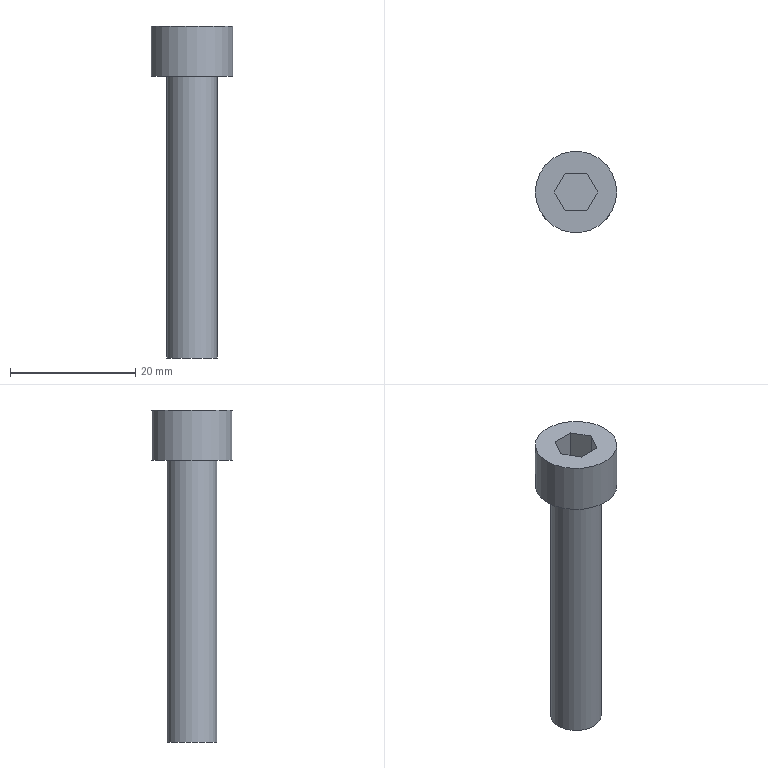Part | STEP file | 1 solid | 12 faces | box 13 x 13 x 53 mm | volume 3159 mm3 | plane 10 | cylinder 2 | commonest cylinder face diameters 8 x1 13 x1
STEP:
#1=CARTESIAN_POINT('',(0.,0.,0.));
#2=DIRECTION('',(0.,0.,1.));
#3=DIRECTION('',(1.,0.,0.));
#4=AXIS2_PLACEMENT_3D('',#1,#2,#3);
#5=CARTESIAN_POINT('',(1566.747,387.48,-61.381));
#6=VERTEX_POINT('',#5);
#7=CARTESIAN_POINT('',(1560.247,387.48,-61.381));
#8=DIRECTION('',(0.,0.,1.));
#9=DIRECTION('',(1.,0.,0.));
#10=AXIS2_PLACEMENT_3D('',#7,#8,#9);
#11=CIRCLE('',#10,6.5);
#12=CARTESIAN_POINT('',(1566.747,387.48,-61.381));
#13=DIRECTION('',(0.,0.,-1.));
#14=DIRECTION('',(-1.,0.,0.));
#15=AXIS2_PLACEMENT_3D('',#12,#13,#14);
#16=PLANE('',#15);
#17=CARTESIAN_POINT('',(0.,0.));
#18=CARTESIAN_POINT('',(0.,11.258));
#19=CARTESIAN_POINT('',(9.75,5.629));
#20=CARTESIAN_POINT('',(19.5,0.));
#21=CARTESIAN_POINT('',(9.75,-5.629));
#22=CARTESIAN_POINT('',(0.,-11.258));
#23=CARTESIAN_POINT('',(0.,0.));
#24=(BOUNDED_CURVE()B_SPLINE_CURVE(2,(#17,#18,#19,#20,#21,#22,#23),.UNSPECIFIED.,.T.,.F.)B_SPLINE_CURVE_WITH_KNOTS((1,2,2,2,2,1),(-2.094,0.,2.094,4.189,6.283,8.378),.UNSPECIFIED.)CURVE()GEOMETRIC_REPRESENTATION_ITEM()RATIONAL_B_SPLINE_CURVE((1.,0.5,1.,0.5,1.,0.5,1.))REPRESENTATION_ITEM(''));
#25=(GEOMETRIC_REPRESENTATION_CONTEXT(2)PARAMETRIC_REPRESENTATION_CONTEXT()REPRESENTATION_CONTEXT('',''));
#26=DEFINITIONAL_REPRESENTATION('',(#24),#25);
#27=PCURVE('',#16,#26);
#28=CARTESIAN_POINT('',(1560.247,387.48,-101.281));
#29=DIRECTION('',(0.,0.,1.));
#30=DIRECTION('',(1.,0.,0.));
#31=AXIS2_PLACEMENT_3D('',#28,#29,#30);
#32=CYLINDRICAL_SURFACE('',#31,6.5);
#33=CARTESIAN_POINT('',(0.,39.9));
#34=DIRECTION('',(1.,0.));
#35=VECTOR('',#34,1.);
#36=LINE('',#33,#35);
#37=(GEOMETRIC_REPRESENTATION_CONTEXT(2)PARAMETRIC_REPRESENTATION_CONTEXT()REPRESENTATION_CONTEXT('',''));
#38=DEFINITIONAL_REPRESENTATION('',(#36),#37);
#39=PCURVE('',#32,#38);
#40=SURFACE_CURVE('',#11,(#27,#39),.PCURVE_S1.);
#41=EDGE_CURVE('',#6,#6,#40,.T.);
#42=ORIENTED_EDGE('',*,*,#41,.T.);
#43=EDGE_LOOP('',(#42));
#44=FACE_BOUND('',#43,.T.);
#45=CARTESIAN_POINT('',(1558.515,390.48,-61.381));
#46=VERTEX_POINT('',#45);
#47=CARTESIAN_POINT('',(1561.979,390.48,-61.381));
#48=VERTEX_POINT('',#47);
#49=CARTESIAN_POINT('',(1558.515,390.48,-61.381));
#50=DIRECTION('',(1.,0.,0.));
#51=VECTOR('',#50,1.);
#52=LINE('',#49,#51);
#53=CARTESIAN_POINT('',(8.232,3.));
#54=DIRECTION('',(-1.,0.));
#55=VECTOR('',#54,1.);
#56=LINE('',#53,#55);
#57=(GEOMETRIC_REPRESENTATION_CONTEXT(2)PARAMETRIC_REPRESENTATION_CONTEXT()REPRESENTATION_CONTEXT('',''));
#58=DEFINITIONAL_REPRESENTATION('',(#56),#57);
#59=PCURVE('',#16,#58);
#60=CARTESIAN_POINT('',(1558.515,390.48,-66.661));
#61=DIRECTION('',(0.,-1.,0.));
#62=DIRECTION('',(1.,0.,0.));
#63=AXIS2_PLACEMENT_3D('',#60,#61,#62);
#64=PLANE('',#63);
#65=CARTESIAN_POINT('',(0.,5.28));
#66=DIRECTION('',(1.,0.));
#67=VECTOR('',#66,1.);
#68=LINE('',#65,#67);
#69=(GEOMETRIC_REPRESENTATION_CONTEXT(2)PARAMETRIC_REPRESENTATION_CONTEXT()REPRESENTATION_CONTEXT('',''));
#70=DEFINITIONAL_REPRESENTATION('',(#68),#69);
#71=PCURVE('',#64,#70);
#72=SURFACE_CURVE('',#52,(#59,#71),.PCURVE_S1.);
#73=EDGE_CURVE('',#46,#48,#72,.T.);
#74=ORIENTED_EDGE('',*,*,#73,.T.);
#75=CARTESIAN_POINT('',(1563.711,387.48,-61.381));
#76=VERTEX_POINT('',#75);
#77=CARTESIAN_POINT('',(1561.979,390.48,-61.381));
#78=DIRECTION('',(0.5,-0.866,0.));
#79=VECTOR('',#78,1.);
#80=LINE('',#77,#79);
#81=CARTESIAN_POINT('',(4.768,3.));
#82=DIRECTION('',(-0.5,-0.866));
#83=VECTOR('',#82,1.);
#84=LINE('',#81,#83);
#85=(GEOMETRIC_REPRESENTATION_CONTEXT(2)PARAMETRIC_REPRESENTATION_CONTEXT()REPRESENTATION_CONTEXT('',''));
#86=DEFINITIONAL_REPRESENTATION('',(#84),#85);
#87=PCURVE('',#16,#86);
#88=CARTESIAN_POINT('',(1561.979,390.48,-66.661));
#89=DIRECTION('',(-0.866,-0.5,0.));
#90=DIRECTION('',(0.5,-0.866,0.));
#91=AXIS2_PLACEMENT_3D('',#88,#89,#90);
#92=PLANE('',#91);
#93=CARTESIAN_POINT('',(0.,5.28));
#94=DIRECTION('',(1.,0.));
#95=VECTOR('',#94,1.);
#96=LINE('',#93,#95);
#97=(GEOMETRIC_REPRESENTATION_CONTEXT(2)PARAMETRIC_REPRESENTATION_CONTEXT()REPRESENTATION_CONTEXT('',''));
#98=DEFINITIONAL_REPRESENTATION('',(#96),#97);
#99=PCURVE('',#92,#98);
#100=SURFACE_CURVE('',#80,(#87,#99),.PCURVE_S1.);
#101=EDGE_CURVE('',#48,#76,#100,.T.);
#102=ORIENTED_EDGE('',*,*,#101,.T.);
#103=CARTESIAN_POINT('',(1561.979,384.48,-61.381));
#104=VERTEX_POINT('',#103);
#105=CARTESIAN_POINT('',(1563.711,387.48,-61.381));
#106=DIRECTION('',(-0.5,-0.866,0.));
#107=VECTOR('',#106,1.);
#108=LINE('',#105,#107);
#109=CARTESIAN_POINT('',(3.036,0.));
#110=DIRECTION('',(0.5,-0.866));
#111=VECTOR('',#110,1.);
#112=LINE('',#109,#111);
#113=(GEOMETRIC_REPRESENTATION_CONTEXT(2)PARAMETRIC_REPRESENTATION_CONTEXT()REPRESENTATION_CONTEXT('',''));
#114=DEFINITIONAL_REPRESENTATION('',(#112),#113);
#115=PCURVE('',#16,#114);
#116=CARTESIAN_POINT('',(1563.711,387.48,-66.661));
#117=DIRECTION('',(-0.866,0.5,0.));
#118=DIRECTION('',(-0.5,-0.866,0.));
#119=AXIS2_PLACEMENT_3D('',#116,#117,#118);
#120=PLANE('',#119);
#121=CARTESIAN_POINT('',(0.,5.28));
#122=DIRECTION('',(1.,0.));
#123=VECTOR('',#122,1.);
#124=LINE('',#121,#123);
#125=(GEOMETRIC_REPRESENTATION_CONTEXT(2)PARAMETRIC_REPRESENTATION_CONTEXT()REPRESENTATION_CONTEXT('',''));
#126=DEFINITIONAL_REPRESENTATION('',(#124),#125);
#127=PCURVE('',#120,#126);
#128=SURFACE_CURVE('',#108,(#115,#127),.PCURVE_S1.);
#129=EDGE_CURVE('',#76,#104,#128,.T.);
#130=ORIENTED_EDGE('',*,*,#129,.T.);
#131=CARTESIAN_POINT('',(1558.515,384.48,-61.381));
#132=VERTEX_POINT('',#131);
#133=CARTESIAN_POINT('',(1561.979,384.48,-61.381));
#134=DIRECTION('',(-1.,0.,0.));
#135=VECTOR('',#134,1.);
#136=LINE('',#133,#135);
#137=CARTESIAN_POINT('',(4.768,-3.));
#138=DIRECTION('',(1.,0.));
#139=VECTOR('',#138,1.);
#140=LINE('',#137,#139);
#141=(GEOMETRIC_REPRESENTATION_CONTEXT(2)PARAMETRIC_REPRESENTATION_CONTEXT()REPRESENTATION_CONTEXT('',''));
#142=DEFINITIONAL_REPRESENTATION('',(#140),#141);
#143=PCURVE('',#16,#142);
#144=CARTESIAN_POINT('',(1561.979,384.48,-66.661));
#145=DIRECTION('',(0.,1.,0.));
#146=DIRECTION('',(-1.,0.,0.));
#147=AXIS2_PLACEMENT_3D('',#144,#145,#146);
#148=PLANE('',#147);
#149=CARTESIAN_POINT('',(0.,5.28));
#150=DIRECTION('',(1.,0.));
#151=VECTOR('',#150,1.);
#152=LINE('',#149,#151);
#153=(GEOMETRIC_REPRESENTATION_CONTEXT(2)PARAMETRIC_REPRESENTATION_CONTEXT()REPRESENTATION_CONTEXT('',''));
#154=DEFINITIONAL_REPRESENTATION('',(#152),#153);
#155=PCURVE('',#148,#154);
#156=SURFACE_CURVE('',#136,(#143,#155),.PCURVE_S1.);
#157=EDGE_CURVE('',#104,#132,#156,.T.);
#158=ORIENTED_EDGE('',*,*,#157,.T.);
#159=CARTESIAN_POINT('',(1556.783,387.48,-61.381));
#160=VERTEX_POINT('',#159);
#161=CARTESIAN_POINT('',(1558.515,384.48,-61.381));
#162=DIRECTION('',(-0.5,0.866,0.));
#163=VECTOR('',#162,1.);
#164=LINE('',#161,#163);
#165=CARTESIAN_POINT('',(8.232,-3.));
#166=DIRECTION('',(0.5,0.866));
#167=VECTOR('',#166,1.);
#168=LINE('',#165,#167);
#169=(GEOMETRIC_REPRESENTATION_CONTEXT(2)PARAMETRIC_REPRESENTATION_CONTEXT()REPRESENTATION_CONTEXT('',''));
#170=DEFINITIONAL_REPRESENTATION('',(#168),#169);
#171=PCURVE('',#16,#170);
#172=CARTESIAN_POINT('',(1558.515,384.48,-66.661));
#173=DIRECTION('',(0.866,0.5,0.));
#174=DIRECTION('',(-0.5,0.866,0.));
#175=AXIS2_PLACEMENT_3D('',#172,#173,#174);
#176=PLANE('',#175);
#177=CARTESIAN_POINT('',(0.,5.28));
#178=DIRECTION('',(1.,0.));
#179=VECTOR('',#178,1.);
#180=LINE('',#177,#179);
#181=(GEOMETRIC_REPRESENTATION_CONTEXT(2)PARAMETRIC_REPRESENTATION_CONTEXT()REPRESENTATION_CONTEXT('',''));
#182=DEFINITIONAL_REPRESENTATION('',(#180),#181);
#183=PCURVE('',#176,#182);
#184=SURFACE_CURVE('',#164,(#171,#183),.PCURVE_S1.);
#185=EDGE_CURVE('',#132,#160,#184,.T.);
#186=ORIENTED_EDGE('',*,*,#185,.T.);
#187=CARTESIAN_POINT('',(1556.783,387.48,-61.381));
#188=DIRECTION('',(0.5,0.866,0.));
#189=VECTOR('',#188,1.);
#190=LINE('',#187,#189);
#191=CARTESIAN_POINT('',(9.964,0.));
#192=DIRECTION('',(-0.5,0.866));
#193=VECTOR('',#192,1.);
#194=LINE('',#191,#193);
#195=(GEOMETRIC_REPRESENTATION_CONTEXT(2)PARAMETRIC_REPRESENTATION_CONTEXT()REPRESENTATION_CONTEXT('',''));
#196=DEFINITIONAL_REPRESENTATION('',(#194),#195);
#197=PCURVE('',#16,#196);
#198=CARTESIAN_POINT('',(1556.783,387.48,-66.661));
#199=DIRECTION('',(0.866,-0.5,0.));
#200=DIRECTION('',(0.5,0.866,0.));
#201=AXIS2_PLACEMENT_3D('',#198,#199,#200);
#202=PLANE('',#201);
#203=CARTESIAN_POINT('',(0.,5.28));
#204=DIRECTION('',(1.,0.));
#205=VECTOR('',#204,1.);
#206=LINE('',#203,#205);
#207=(GEOMETRIC_REPRESENTATION_CONTEXT(2)PARAMETRIC_REPRESENTATION_CONTEXT()REPRESENTATION_CONTEXT('',''));
#208=DEFINITIONAL_REPRESENTATION('',(#206),#207);
#209=PCURVE('',#202,#208);
#210=SURFACE_CURVE('',#190,(#197,#209),.PCURVE_S1.);
#211=EDGE_CURVE('',#160,#46,#210,.T.);
#212=ORIENTED_EDGE('',*,*,#211,.T.);
#213=EDGE_LOOP('',(#74,#102,#130,#158,#186,#212));
#214=FACE_BOUND('',#213,.T.);
#215=ADVANCED_FACE('',(#44,#214),#16,.F.);
#216=ORIENTED_EDGE('',*,*,#41,.F.);
#217=CARTESIAN_POINT('',(1566.747,387.48,-69.381));
#218=VERTEX_POINT('',#217);
#219=CARTESIAN_POINT('',(1566.747,387.48,-69.381));
#220=CARTESIAN_POINT('',(1566.747,387.48,-61.381));
#221=B_SPLINE_CURVE_WITH_KNOTS('',1,(#219,#220),.UNSPECIFIED.,.F.,.F.,(2,2),(31.9,39.9),.PIECEWISE_BEZIER_KNOTS.);
#222=CARTESIAN_POINT('',(0.,0.));
#223=DIRECTION('',(0.,1.));
#224=VECTOR('',#223,1.);
#225=LINE('',#222,#224);
#226=(GEOMETRIC_REPRESENTATION_CONTEXT(2)PARAMETRIC_REPRESENTATION_CONTEXT()REPRESENTATION_CONTEXT('',''));
#227=DEFINITIONAL_REPRESENTATION('',(#225),#226);
#228=PCURVE('',#32,#227);
#229=CARTESIAN_POINT('',(6.283,0.));
#230=DIRECTION('',(0.,1.));
#231=VECTOR('',#230,1.);
#232=LINE('',#229,#231);
#233=(GEOMETRIC_REPRESENTATION_CONTEXT(2)PARAMETRIC_REPRESENTATION_CONTEXT()REPRESENTATION_CONTEXT('',''));
#234=DEFINITIONAL_REPRESENTATION('',(#232),#233);
#235=PCURVE('',#32,#234);
#236=SEAM_CURVE('',#221,(#228,#235),.PCURVE_S1.);
#237=EDGE_CURVE('',#218,#6,#236,.T.);
#238=ORIENTED_EDGE('',*,*,#237,.F.);
#239=CARTESIAN_POINT('',(1560.247,387.48,-69.381));
#240=DIRECTION('',(0.,0.,1.));
#241=DIRECTION('',(1.,0.,0.));
#242=AXIS2_PLACEMENT_3D('',#239,#240,#241);
#243=CIRCLE('',#242,6.5);
#244=CARTESIAN_POINT('',(0.,31.9));
#245=DIRECTION('',(1.,0.));
#246=VECTOR('',#245,1.);
#247=LINE('',#244,#246);
#248=(GEOMETRIC_REPRESENTATION_CONTEXT(2)PARAMETRIC_REPRESENTATION_CONTEXT()REPRESENTATION_CONTEXT('',''));
#249=DEFINITIONAL_REPRESENTATION('',(#247),#248);
#250=PCURVE('',#32,#249);
#251=CARTESIAN_POINT('',(1564.247,387.48,-69.381));
#252=DIRECTION('',(0.,0.,1.));
#253=DIRECTION('',(1.,0.,0.));
#254=AXIS2_PLACEMENT_3D('',#251,#252,#253);
#255=PLANE('',#254);
#256=CARTESIAN_POINT('',(-4.,0.));
#257=DIRECTION('',(1.,0.));
#258=AXIS2_PLACEMENT_2D('',#256,#257);
#259=CIRCLE('',#258,6.5);
#260=(GEOMETRIC_REPRESENTATION_CONTEXT(2)PARAMETRIC_REPRESENTATION_CONTEXT()REPRESENTATION_CONTEXT('',''));
#261=DEFINITIONAL_REPRESENTATION('',(#259),#260);
#262=PCURVE('',#255,#261);
#263=SURFACE_CURVE('',#243,(#250,#262),.PCURVE_S1.);
#264=EDGE_CURVE('',#218,#218,#263,.T.);
#265=ORIENTED_EDGE('',*,*,#264,.T.);
#266=ORIENTED_EDGE('',*,*,#237,.T.);
#267=EDGE_LOOP('',(#216,#238,#265,#266));
#268=FACE_BOUND('',#267,.T.);
#269=ADVANCED_FACE('',(#268),#32,.T.);
#270=ORIENTED_EDGE('',*,*,#264,.F.);
#271=EDGE_LOOP('',(#270));
#272=FACE_BOUND('',#271,.T.);
#273=CARTESIAN_POINT('',(1564.247,387.48,-69.381));
#274=VERTEX_POINT('',#273);
#275=CARTESIAN_POINT('',(1560.247,387.48,-69.381));
#276=DIRECTION('',(0.,0.,1.));
#277=DIRECTION('',(1.,0.,0.));
#278=AXIS2_PLACEMENT_3D('',#275,#276,#277);
#279=CIRCLE('',#278,4.);
#280=CARTESIAN_POINT('',(-4.,0.));
#281=DIRECTION('',(1.,0.));
#282=AXIS2_PLACEMENT_2D('',#280,#281);
#283=CIRCLE('',#282,4.);
#284=(GEOMETRIC_REPRESENTATION_CONTEXT(2)PARAMETRIC_REPRESENTATION_CONTEXT()REPRESENTATION_CONTEXT('',''));
#285=DEFINITIONAL_REPRESENTATION('',(#283),#284);
#286=PCURVE('',#255,#285);
#287=CARTESIAN_POINT('',(1560.247,387.48,-101.281));
#288=DIRECTION('',(0.,0.,1.));
#289=DIRECTION('',(1.,0.,0.));
#290=AXIS2_PLACEMENT_3D('',#287,#288,#289);
#291=CYLINDRICAL_SURFACE('',#290,4.);
#292=CARTESIAN_POINT('',(0.,31.9));
#293=DIRECTION('',(1.,0.));
#294=VECTOR('',#293,1.);
#295=LINE('',#292,#294);
#296=(GEOMETRIC_REPRESENTATION_CONTEXT(2)PARAMETRIC_REPRESENTATION_CONTEXT()REPRESENTATION_CONTEXT('',''));
#297=DEFINITIONAL_REPRESENTATION('',(#295),#296);
#298=PCURVE('',#291,#297);
#299=SURFACE_CURVE('',#279,(#286,#298),.PCURVE_S1.);
#300=EDGE_CURVE('',#274,#274,#299,.T.);
#301=ORIENTED_EDGE('',*,*,#300,.T.);
#302=EDGE_LOOP('',(#301));
#303=FACE_BOUND('',#302,.T.);
#304=ADVANCED_FACE('',(#272,#303),#255,.F.);
#305=ORIENTED_EDGE('',*,*,#300,.F.);
#306=CARTESIAN_POINT('',(1564.247,387.48,-114.381));
#307=VERTEX_POINT('',#306);
#308=CARTESIAN_POINT('',(1564.247,387.48,-114.381));
#309=CARTESIAN_POINT('',(1564.247,387.48,-69.381));
#310=B_SPLINE_CURVE_WITH_KNOTS('',1,(#308,#309),.UNSPECIFIED.,.F.,.F.,(2,2),(-13.1,31.9),.PIECEWISE_BEZIER_KNOTS.);
#311=CARTESIAN_POINT('',(0.,0.));
#312=DIRECTION('',(0.,1.));
#313=VECTOR('',#312,1.);
#314=LINE('',#311,#313);
#315=(GEOMETRIC_REPRESENTATION_CONTEXT(2)PARAMETRIC_REPRESENTATION_CONTEXT()REPRESENTATION_CONTEXT('',''));
#316=DEFINITIONAL_REPRESENTATION('',(#314),#315);
#317=PCURVE('',#291,#316);
#318=CARTESIAN_POINT('',(6.283,0.));
#319=DIRECTION('',(0.,1.));
#320=VECTOR('',#319,1.);
#321=LINE('',#318,#320);
#322=(GEOMETRIC_REPRESENTATION_CONTEXT(2)PARAMETRIC_REPRESENTATION_CONTEXT()REPRESENTATION_CONTEXT('',''));
#323=DEFINITIONAL_REPRESENTATION('',(#321),#322);
#324=PCURVE('',#291,#323);
#325=SEAM_CURVE('',#310,(#317,#324),.PCURVE_S1.);
#326=EDGE_CURVE('',#307,#274,#325,.T.);
#327=ORIENTED_EDGE('',*,*,#326,.F.);
#328=CARTESIAN_POINT('',(1560.247,387.48,-114.381));
#329=DIRECTION('',(0.,0.,1.));
#330=DIRECTION('',(1.,0.,0.));
#331=AXIS2_PLACEMENT_3D('',#328,#329,#330);
#332=CIRCLE('',#331,4.);
#333=CARTESIAN_POINT('',(0.,-13.1));
#334=DIRECTION('',(1.,0.));
#335=VECTOR('',#334,1.);
#336=LINE('',#333,#335);
#337=(GEOMETRIC_REPRESENTATION_CONTEXT(2)PARAMETRIC_REPRESENTATION_CONTEXT()REPRESENTATION_CONTEXT('',''));
#338=DEFINITIONAL_REPRESENTATION('',(#336),#337);
#339=PCURVE('',#291,#338);
#340=CARTESIAN_POINT('',(1560.247,387.48,-114.381));
#341=DIRECTION('',(0.,0.,1.));
#342=DIRECTION('',(1.,0.,0.));
#343=AXIS2_PLACEMENT_3D('',#340,#341,#342);
#344=PLANE('',#343);
#345=CARTESIAN_POINT('',(0.,0.));
#346=DIRECTION('',(1.,0.));
#347=AXIS2_PLACEMENT_2D('',#345,#346);
#348=CIRCLE('',#347,4.);
#349=(GEOMETRIC_REPRESENTATION_CONTEXT(2)PARAMETRIC_REPRESENTATION_CONTEXT()REPRESENTATION_CONTEXT('',''));
#350=DEFINITIONAL_REPRESENTATION('',(#348),#349);
#351=PCURVE('',#344,#350);
#352=SURFACE_CURVE('',#332,(#339,#351),.PCURVE_S1.);
#353=EDGE_CURVE('',#307,#307,#352,.T.);
#354=ORIENTED_EDGE('',*,*,#353,.T.);
#355=ORIENTED_EDGE('',*,*,#326,.T.);
#356=EDGE_LOOP('',(#305,#327,#354,#355));
#357=FACE_BOUND('',#356,.T.);
#358=ADVANCED_FACE('',(#357),#291,.T.);
#359=ORIENTED_EDGE('',*,*,#353,.F.);
#360=EDGE_LOOP('',(#359));
#361=FACE_BOUND('',#360,.T.);
#362=ADVANCED_FACE('',(#361),#344,.F.);
#363=ORIENTED_EDGE('',*,*,#73,.F.);
#364=CARTESIAN_POINT('',(1558.515,390.48,-66.661));
#365=VERTEX_POINT('',#364);
#366=CARTESIAN_POINT('',(1558.515,390.48,-66.661));
#367=DIRECTION('',(0.,0.,-1.));
#368=VECTOR('',#367,1.);
#369=LINE('',#366,#368);
#370=CARTESIAN_POINT('',(0.,0.));
#371=DIRECTION('',(0.,-1.));
#372=VECTOR('',#371,1.);
#373=LINE('',#370,#372);
#374=(GEOMETRIC_REPRESENTATION_CONTEXT(2)PARAMETRIC_REPRESENTATION_CONTEXT()REPRESENTATION_CONTEXT('',''));
#375=DEFINITIONAL_REPRESENTATION('',(#373),#374);
#376=PCURVE('',#64,#375);
#377=CARTESIAN_POINT('',(3.464,0.));
#378=DIRECTION('',(0.,-1.));
#379=VECTOR('',#378,1.);
#380=LINE('',#377,#379);
#381=(GEOMETRIC_REPRESENTATION_CONTEXT(2)PARAMETRIC_REPRESENTATION_CONTEXT()REPRESENTATION_CONTEXT('',''));
#382=DEFINITIONAL_REPRESENTATION('',(#380),#381);
#383=PCURVE('',#202,#382);
#384=SURFACE_CURVE('',#369,(#376,#383),.PCURVE_S1.);
#385=EDGE_CURVE('',#46,#365,#384,.T.);
#386=ORIENTED_EDGE('',*,*,#385,.T.);
#387=CARTESIAN_POINT('',(1561.979,390.48,-66.661));
#388=VERTEX_POINT('',#387);
#389=CARTESIAN_POINT('',(1558.515,390.48,-66.661));
#390=DIRECTION('',(-1.,0.,0.));
#391=VECTOR('',#390,1.);
#392=LINE('',#389,#391);
#393=CARTESIAN_POINT('',(0.,0.));
#394=DIRECTION('',(-1.,0.));
#395=VECTOR('',#394,1.);
#396=LINE('',#393,#395);
#397=(GEOMETRIC_REPRESENTATION_CONTEXT(2)PARAMETRIC_REPRESENTATION_CONTEXT()REPRESENTATION_CONTEXT('',''));
#398=DEFINITIONAL_REPRESENTATION('',(#396),#397);
#399=PCURVE('',#64,#398);
#400=CARTESIAN_POINT('',(1560.247,387.48,-66.661));
#401=DIRECTION('',(0.,0.,-1.));
#402=DIRECTION('',(-1.,0.,0.));
#403=AXIS2_PLACEMENT_3D('',#400,#401,#402);
#404=PLANE('',#403);
#405=CARTESIAN_POINT('',(1.732,3.));
#406=DIRECTION('',(1.,0.));
#407=VECTOR('',#406,1.);
#408=LINE('',#405,#407);
#409=(GEOMETRIC_REPRESENTATION_CONTEXT(2)PARAMETRIC_REPRESENTATION_CONTEXT()REPRESENTATION_CONTEXT('',''));
#410=DEFINITIONAL_REPRESENTATION('',(#408),#409);
#411=PCURVE('',#404,#410);
#412=SURFACE_CURVE('',#392,(#399,#411),.PCURVE_S1.);
#413=EDGE_CURVE('',#388,#365,#412,.T.);
#414=ORIENTED_EDGE('',*,*,#413,.F.);
#415=CARTESIAN_POINT('',(1561.979,390.48,-66.661));
#416=DIRECTION('',(0.,0.,-1.));
#417=VECTOR('',#416,1.);
#418=LINE('',#415,#417);
#419=CARTESIAN_POINT('',(3.464,0.));
#420=DIRECTION('',(0.,-1.));
#421=VECTOR('',#420,1.);
#422=LINE('',#419,#421);
#423=(GEOMETRIC_REPRESENTATION_CONTEXT(2)PARAMETRIC_REPRESENTATION_CONTEXT()REPRESENTATION_CONTEXT('',''));
#424=DEFINITIONAL_REPRESENTATION('',(#422),#423);
#425=PCURVE('',#64,#424);
#426=CARTESIAN_POINT('',(0.,0.));
#427=DIRECTION('',(0.,-1.));
#428=VECTOR('',#427,1.);
#429=LINE('',#426,#428);
#430=(GEOMETRIC_REPRESENTATION_CONTEXT(2)PARAMETRIC_REPRESENTATION_CONTEXT()REPRESENTATION_CONTEXT('',''));
#431=DEFINITIONAL_REPRESENTATION('',(#429),#430);
#432=PCURVE('',#92,#431);
#433=SURFACE_CURVE('',#418,(#425,#432),.PCURVE_S1.);
#434=EDGE_CURVE('',#48,#388,#433,.T.);
#435=ORIENTED_EDGE('',*,*,#434,.F.);
#436=EDGE_LOOP('',(#363,#386,#414,#435));
#437=FACE_BOUND('',#436,.T.);
#438=ADVANCED_FACE('',(#437),#64,.T.);
#439=ORIENTED_EDGE('',*,*,#101,.F.);
#440=ORIENTED_EDGE('',*,*,#434,.T.);
#441=CARTESIAN_POINT('',(1563.711,387.48,-66.661));
#442=VERTEX_POINT('',#441);
#443=CARTESIAN_POINT('',(1561.979,390.48,-66.661));
#444=DIRECTION('',(-0.5,0.866,0.));
#445=VECTOR('',#444,1.);
#446=LINE('',#443,#445);
#447=CARTESIAN_POINT('',(0.,0.));
#448=DIRECTION('',(-1.,0.));
#449=VECTOR('',#448,1.);
#450=LINE('',#447,#449);
#451=(GEOMETRIC_REPRESENTATION_CONTEXT(2)PARAMETRIC_REPRESENTATION_CONTEXT()REPRESENTATION_CONTEXT('',''));
#452=DEFINITIONAL_REPRESENTATION('',(#450),#451);
#453=PCURVE('',#92,#452);
#454=CARTESIAN_POINT('',(-1.732,3.));
#455=DIRECTION('',(0.5,0.866));
#456=VECTOR('',#455,1.);
#457=LINE('',#454,#456);
#458=(GEOMETRIC_REPRESENTATION_CONTEXT(2)PARAMETRIC_REPRESENTATION_CONTEXT()REPRESENTATION_CONTEXT('',''));
#459=DEFINITIONAL_REPRESENTATION('',(#457),#458);
#460=PCURVE('',#404,#459);
#461=SURFACE_CURVE('',#446,(#453,#460),.PCURVE_S1.);
#462=EDGE_CURVE('',#442,#388,#461,.T.);
#463=ORIENTED_EDGE('',*,*,#462,.F.);
#464=CARTESIAN_POINT('',(1563.711,387.48,-66.661));
#465=DIRECTION('',(0.,0.,-1.));
#466=VECTOR('',#465,1.);
#467=LINE('',#464,#466);
#468=CARTESIAN_POINT('',(3.464,0.));
#469=DIRECTION('',(0.,-1.));
#470=VECTOR('',#469,1.);
#471=LINE('',#468,#470);
#472=(GEOMETRIC_REPRESENTATION_CONTEXT(2)PARAMETRIC_REPRESENTATION_CONTEXT()REPRESENTATION_CONTEXT('',''));
#473=DEFINITIONAL_REPRESENTATION('',(#471),#472);
#474=PCURVE('',#92,#473);
#475=CARTESIAN_POINT('',(0.,0.));
#476=DIRECTION('',(0.,-1.));
#477=VECTOR('',#476,1.);
#478=LINE('',#475,#477);
#479=(GEOMETRIC_REPRESENTATION_CONTEXT(2)PARAMETRIC_REPRESENTATION_CONTEXT()REPRESENTATION_CONTEXT('',''));
#480=DEFINITIONAL_REPRESENTATION('',(#478),#479);
#481=PCURVE('',#120,#480);
#482=SURFACE_CURVE('',#467,(#474,#481),.PCURVE_S1.);
#483=EDGE_CURVE('',#76,#442,#482,.T.);
#484=ORIENTED_EDGE('',*,*,#483,.F.);
#485=EDGE_LOOP('',(#439,#440,#463,#484));
#486=FACE_BOUND('',#485,.T.);
#487=ADVANCED_FACE('',(#486),#92,.T.);
#488=ORIENTED_EDGE('',*,*,#129,.F.);
#489=ORIENTED_EDGE('',*,*,#483,.T.);
#490=CARTESIAN_POINT('',(1561.979,384.48,-66.661));
#491=VERTEX_POINT('',#490);
#492=CARTESIAN_POINT('',(1563.711,387.48,-66.661));
#493=DIRECTION('',(0.5,0.866,0.));
#494=VECTOR('',#493,1.);
#495=LINE('',#492,#494);
#496=CARTESIAN_POINT('',(0.,0.));
#497=DIRECTION('',(-1.,0.));
#498=VECTOR('',#497,1.);
#499=LINE('',#496,#498);
#500=(GEOMETRIC_REPRESENTATION_CONTEXT(2)PARAMETRIC_REPRESENTATION_CONTEXT()REPRESENTATION_CONTEXT('',''));
#501=DEFINITIONAL_REPRESENTATION('',(#499),#500);
#502=PCURVE('',#120,#501);
#503=CARTESIAN_POINT('',(-3.464,0.));
#504=DIRECTION('',(-0.5,0.866));
#505=VECTOR('',#504,1.);
#506=LINE('',#503,#505);
#507=(GEOMETRIC_REPRESENTATION_CONTEXT(2)PARAMETRIC_REPRESENTATION_CONTEXT()REPRESENTATION_CONTEXT('',''));
#508=DEFINITIONAL_REPRESENTATION('',(#506),#507);
#509=PCURVE('',#404,#508);
#510=SURFACE_CURVE('',#495,(#502,#509),.PCURVE_S1.);
#511=EDGE_CURVE('',#491,#442,#510,.T.);
#512=ORIENTED_EDGE('',*,*,#511,.F.);
#513=CARTESIAN_POINT('',(1561.979,384.48,-66.661));
#514=DIRECTION('',(0.,0.,-1.));
#515=VECTOR('',#514,1.);
#516=LINE('',#513,#515);
#517=CARTESIAN_POINT('',(3.464,0.));
#518=DIRECTION('',(0.,-1.));
#519=VECTOR('',#518,1.);
#520=LINE('',#517,#519);
#521=(GEOMETRIC_REPRESENTATION_CONTEXT(2)PARAMETRIC_REPRESENTATION_CONTEXT()REPRESENTATION_CONTEXT('',''));
#522=DEFINITIONAL_REPRESENTATION('',(#520),#521);
#523=PCURVE('',#120,#522);
#524=CARTESIAN_POINT('',(0.,0.));
#525=DIRECTION('',(0.,-1.));
#526=VECTOR('',#525,1.);
#527=LINE('',#524,#526);
#528=(GEOMETRIC_REPRESENTATION_CONTEXT(2)PARAMETRIC_REPRESENTATION_CONTEXT()REPRESENTATION_CONTEXT('',''));
#529=DEFINITIONAL_REPRESENTATION('',(#527),#528);
#530=PCURVE('',#148,#529);
#531=SURFACE_CURVE('',#516,(#523,#530),.PCURVE_S1.);
#532=EDGE_CURVE('',#104,#491,#531,.T.);
#533=ORIENTED_EDGE('',*,*,#532,.F.);
#534=EDGE_LOOP('',(#488,#489,#512,#533));
#535=FACE_BOUND('',#534,.T.);
#536=ADVANCED_FACE('',(#535),#120,.T.);
#537=ORIENTED_EDGE('',*,*,#157,.F.);
#538=ORIENTED_EDGE('',*,*,#532,.T.);
#539=CARTESIAN_POINT('',(1558.515,384.48,-66.661));
#540=VERTEX_POINT('',#539);
#541=CARTESIAN_POINT('',(1561.979,384.48,-66.661));
#542=DIRECTION('',(1.,0.,0.));
#543=VECTOR('',#542,1.);
#544=LINE('',#541,#543);
#545=CARTESIAN_POINT('',(0.,0.));
#546=DIRECTION('',(-1.,0.));
#547=VECTOR('',#546,1.);
#548=LINE('',#545,#547);
#549=(GEOMETRIC_REPRESENTATION_CONTEXT(2)PARAMETRIC_REPRESENTATION_CONTEXT()REPRESENTATION_CONTEXT('',''));
#550=DEFINITIONAL_REPRESENTATION('',(#548),#549);
#551=PCURVE('',#148,#550);
#552=CARTESIAN_POINT('',(-1.732,-3.));
#553=DIRECTION('',(-1.,0.));
#554=VECTOR('',#553,1.);
#555=LINE('',#552,#554);
#556=(GEOMETRIC_REPRESENTATION_CONTEXT(2)PARAMETRIC_REPRESENTATION_CONTEXT()REPRESENTATION_CONTEXT('',''));
#557=DEFINITIONAL_REPRESENTATION('',(#555),#556);
#558=PCURVE('',#404,#557);
#559=SURFACE_CURVE('',#544,(#551,#558),.PCURVE_S1.);
#560=EDGE_CURVE('',#540,#491,#559,.T.);
#561=ORIENTED_EDGE('',*,*,#560,.F.);
#562=CARTESIAN_POINT('',(1558.515,384.48,-66.661));
#563=DIRECTION('',(0.,0.,-1.));
#564=VECTOR('',#563,1.);
#565=LINE('',#562,#564);
#566=CARTESIAN_POINT('',(3.464,0.));
#567=DIRECTION('',(0.,-1.));
#568=VECTOR('',#567,1.);
#569=LINE('',#566,#568);
#570=(GEOMETRIC_REPRESENTATION_CONTEXT(2)PARAMETRIC_REPRESENTATION_CONTEXT()REPRESENTATION_CONTEXT('',''));
#571=DEFINITIONAL_REPRESENTATION('',(#569),#570);
#572=PCURVE('',#148,#571);
#573=CARTESIAN_POINT('',(0.,0.));
#574=DIRECTION('',(0.,-1.));
#575=VECTOR('',#574,1.);
#576=LINE('',#573,#575);
#577=(GEOMETRIC_REPRESENTATION_CONTEXT(2)PARAMETRIC_REPRESENTATION_CONTEXT()REPRESENTATION_CONTEXT('',''));
#578=DEFINITIONAL_REPRESENTATION('',(#576),#577);
#579=PCURVE('',#176,#578);
#580=SURFACE_CURVE('',#565,(#572,#579),.PCURVE_S1.);
#581=EDGE_CURVE('',#132,#540,#580,.T.);
#582=ORIENTED_EDGE('',*,*,#581,.F.);
#583=EDGE_LOOP('',(#537,#538,#561,#582));
#584=FACE_BOUND('',#583,.T.);
#585=ADVANCED_FACE('',(#584),#148,.T.);
#586=ORIENTED_EDGE('',*,*,#185,.F.);
#587=ORIENTED_EDGE('',*,*,#581,.T.);
#588=CARTESIAN_POINT('',(1556.783,387.48,-66.661));
#589=VERTEX_POINT('',#588);
#590=CARTESIAN_POINT('',(1558.515,384.48,-66.661));
#591=DIRECTION('',(0.5,-0.866,0.));
#592=VECTOR('',#591,1.);
#593=LINE('',#590,#592);
#594=CARTESIAN_POINT('',(0.,0.));
#595=DIRECTION('',(-1.,0.));
#596=VECTOR('',#595,1.);
#597=LINE('',#594,#596);
#598=(GEOMETRIC_REPRESENTATION_CONTEXT(2)PARAMETRIC_REPRESENTATION_CONTEXT()REPRESENTATION_CONTEXT('',''));
#599=DEFINITIONAL_REPRESENTATION('',(#597),#598);
#600=PCURVE('',#176,#599);
#601=CARTESIAN_POINT('',(1.732,-3.));
#602=DIRECTION('',(-0.5,-0.866));
#603=VECTOR('',#602,1.);
#604=LINE('',#601,#603);
#605=(GEOMETRIC_REPRESENTATION_CONTEXT(2)PARAMETRIC_REPRESENTATION_CONTEXT()REPRESENTATION_CONTEXT('',''));
#606=DEFINITIONAL_REPRESENTATION('',(#604),#605);
#607=PCURVE('',#404,#606);
#608=SURFACE_CURVE('',#593,(#600,#607),.PCURVE_S1.);
#609=EDGE_CURVE('',#589,#540,#608,.T.);
#610=ORIENTED_EDGE('',*,*,#609,.F.);
#611=CARTESIAN_POINT('',(1556.783,387.48,-66.661));
#612=DIRECTION('',(0.,0.,-1.));
#613=VECTOR('',#612,1.);
#614=LINE('',#611,#613);
#615=CARTESIAN_POINT('',(3.464,0.));
#616=DIRECTION('',(0.,-1.));
#617=VECTOR('',#616,1.);
#618=LINE('',#615,#617);
#619=(GEOMETRIC_REPRESENTATION_CONTEXT(2)PARAMETRIC_REPRESENTATION_CONTEXT()REPRESENTATION_CONTEXT('',''));
#620=DEFINITIONAL_REPRESENTATION('',(#618),#619);
#621=PCURVE('',#176,#620);
#622=CARTESIAN_POINT('',(0.,0.));
#623=DIRECTION('',(0.,-1.));
#624=VECTOR('',#623,1.);
#625=LINE('',#622,#624);
#626=(GEOMETRIC_REPRESENTATION_CONTEXT(2)PARAMETRIC_REPRESENTATION_CONTEXT()REPRESENTATION_CONTEXT('',''));
#627=DEFINITIONAL_REPRESENTATION('',(#625),#626);
#628=PCURVE('',#202,#627);
#629=SURFACE_CURVE('',#614,(#621,#628),.PCURVE_S1.);
#630=EDGE_CURVE('',#160,#589,#629,.T.);
#631=ORIENTED_EDGE('',*,*,#630,.F.);
#632=EDGE_LOOP('',(#586,#587,#610,#631));
#633=FACE_BOUND('',#632,.T.);
#634=ADVANCED_FACE('',(#633),#176,.T.);
#635=ORIENTED_EDGE('',*,*,#211,.F.);
#636=ORIENTED_EDGE('',*,*,#630,.T.);
#637=CARTESIAN_POINT('',(1556.783,387.48,-66.661));
#638=DIRECTION('',(-0.5,-0.866,0.));
#639=VECTOR('',#638,1.);
#640=LINE('',#637,#639);
#641=CARTESIAN_POINT('',(0.,0.));
#642=DIRECTION('',(-1.,0.));
#643=VECTOR('',#642,1.);
#644=LINE('',#641,#643);
#645=(GEOMETRIC_REPRESENTATION_CONTEXT(2)PARAMETRIC_REPRESENTATION_CONTEXT()REPRESENTATION_CONTEXT('',''));
#646=DEFINITIONAL_REPRESENTATION('',(#644),#645);
#647=PCURVE('',#202,#646);
#648=CARTESIAN_POINT('',(3.464,0.));
#649=DIRECTION('',(0.5,-0.866));
#650=VECTOR('',#649,1.);
#651=LINE('',#648,#650);
#652=(GEOMETRIC_REPRESENTATION_CONTEXT(2)PARAMETRIC_REPRESENTATION_CONTEXT()REPRESENTATION_CONTEXT('',''));
#653=DEFINITIONAL_REPRESENTATION('',(#651),#652);
#654=PCURVE('',#404,#653);
#655=SURFACE_CURVE('',#640,(#647,#654),.PCURVE_S1.);
#656=EDGE_CURVE('',#365,#589,#655,.T.);
#657=ORIENTED_EDGE('',*,*,#656,.F.);
#658=ORIENTED_EDGE('',*,*,#385,.F.);
#659=EDGE_LOOP('',(#635,#636,#657,#658));
#660=FACE_BOUND('',#659,.T.);
#661=ADVANCED_FACE('',(#660),#202,.T.);
#662=ORIENTED_EDGE('',*,*,#413,.T.);
#663=ORIENTED_EDGE('',*,*,#656,.T.);
#664=ORIENTED_EDGE('',*,*,#609,.T.);
#665=ORIENTED_EDGE('',*,*,#560,.T.);
#666=ORIENTED_EDGE('',*,*,#511,.T.);
#667=ORIENTED_EDGE('',*,*,#462,.T.);
#668=EDGE_LOOP('',(#662,#663,#664,#665,#666,#667));
#669=FACE_BOUND('',#668,.T.);
#670=ADVANCED_FACE('',(#669),#404,.F.);
#671=CLOSED_SHELL('',(#215,#269,#304,#358,#362,#438,#487,#536,#585,#634,#661,#670));
#672=MANIFOLD_SOLID_BREP('',#671);
#673=(LENGTH_UNIT()NAMED_UNIT(*)SI_UNIT(.MILLI.,.METRE.));
#674=UNCERTAINTY_MEASURE_WITH_UNIT(LENGTH_MEASURE(0.000002),#673,'','');
#675=(NAMED_UNIT(*)PLANE_ANGLE_UNIT()SI_UNIT($,.RADIAN.));
#676=(NAMED_UNIT(*)SI_UNIT($,.STERADIAN.)SOLID_ANGLE_UNIT());
#677=(GEOMETRIC_REPRESENTATION_CONTEXT(3)GLOBAL_UNCERTAINTY_ASSIGNED_CONTEXT((#674))GLOBAL_UNIT_ASSIGNED_CONTEXT((#673,#675,#676))REPRESENTATION_CONTEXT('',''));
#678=ADVANCED_BREP_SHAPE_REPRESENTATION('',(#4,#672),#677);